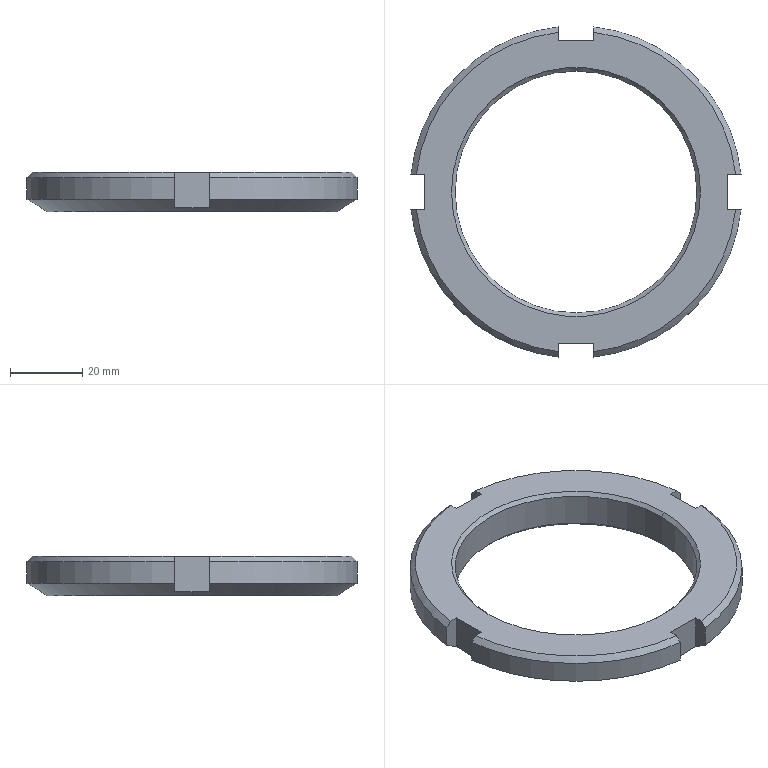Part | SolidWorks | features Chamfer 3, CirPattern 1, Cut 1, Extrusion 1 | 1 solid | 30 faces | box 91.477 x 91.477 x 11 mm | volume 29647 mm3 | plane 14 | cone 10 | cylinder 6 | commonest cylinder face diameters 92 x4 67 x2
STEP:
#1=CARTESIAN_POINT('',(-33.5,0.,10.));
#2=VERTEX_POINT('',#1);
#3=CARTESIAN_POINT('',(33.5,0.,10.));
#4=VERTEX_POINT('',#3);
#5=CARTESIAN_POINT('',(0.,0.,10.));
#6=DIRECTION('',(0.,0.,1.));
#7=DIRECTION('',(1.,0.,0.));
#8=AXIS2_PLACEMENT_3D('',#5,#6,#7);
#9=CIRCLE('',#8,33.5);
#10=EDGE_CURVE('',#2,#4,#9,.T.);
#11=ORIENTED_EDGE('',*,*,#10,.F.);
#12=CARTESIAN_POINT('',(-34.5,0.,11.));
#13=VERTEX_POINT('',#12);
#14=CARTESIAN_POINT('',(-33.5,0.,10.));
#15=DIRECTION('',(-0.7071,0.,0.7071));
#16=VECTOR('',#15,1000.);
#17=LINE('',#14,#16);
#18=EDGE_CURVE('',#2,#13,#17,.T.);
#19=ORIENTED_EDGE('',*,*,#18,.T.);
#20=CARTESIAN_POINT('',(34.5,0.,11.));
#21=VERTEX_POINT('',#20);
#22=CARTESIAN_POINT('',(0.,0.,11.));
#23=DIRECTION('',(0.,0.,-1.));
#24=DIRECTION('',(1.,0.,0.));
#25=AXIS2_PLACEMENT_3D('',#22,#23,#24);
#26=CIRCLE('',#25,34.5);
#27=EDGE_CURVE('',#21,#13,#26,.T.);
#28=ORIENTED_EDGE('',*,*,#27,.F.);
#29=CARTESIAN_POINT('',(33.5,0.,10.));
#30=DIRECTION('',(0.7071,0.,0.7071));
#31=VECTOR('',#30,1000.);
#32=LINE('',#29,#31);
#33=EDGE_CURVE('',#4,#21,#32,.T.);
#34=ORIENTED_EDGE('',*,*,#33,.F.);
#35=EDGE_LOOP('',(#11,#19,#28,#34));
#36=FACE_OUTER_BOUND('',#35,.T.);
#37=CARTESIAN_POINT('',(0.,0.,10.));
#38=DIRECTION('',(0.,0.,1.));
#39=DIRECTION('',(1.,0.,0.));
#40=AXIS2_PLACEMENT_3D('',#37,#38,#39);
#41=CONICAL_SURFACE('',#40,33.5,0.7854);
#42=ADVANCED_FACE('',(#36),#41,.F.);
#43=CARTESIAN_POINT('',(33.5,0.,1.));
#44=VERTEX_POINT('',#43);
#45=CARTESIAN_POINT('',(-33.5,0.,1.));
#46=VERTEX_POINT('',#45);
#47=CARTESIAN_POINT('',(0.,0.,1.));
#48=DIRECTION('',(0.,0.,-1.));
#49=DIRECTION('',(1.,0.,0.));
#50=AXIS2_PLACEMENT_3D('',#47,#48,#49);
#51=CIRCLE('',#50,33.5);
#52=EDGE_CURVE('',#44,#46,#51,.T.);
#53=ORIENTED_EDGE('',*,*,#52,.F.);
#54=CARTESIAN_POINT('',(34.5,0.,0.));
#55=VERTEX_POINT('',#54);
#56=CARTESIAN_POINT('',(34.5,0.,0.));
#57=DIRECTION('',(0.7071,0.,-0.7071));
#58=VECTOR('',#57,1000.);
#59=LINE('',#56,#58);
#60=EDGE_CURVE('',#44,#55,#59,.T.);
#61=ORIENTED_EDGE('',*,*,#60,.T.);
#62=CARTESIAN_POINT('',(-34.5,0.,0.));
#63=VERTEX_POINT('',#62);
#64=CARTESIAN_POINT('',(0.,0.,0.));
#65=DIRECTION('',(0.,0.,1.));
#66=DIRECTION('',(1.,0.,0.));
#67=AXIS2_PLACEMENT_3D('',#64,#65,#66);
#68=CIRCLE('',#67,34.5);
#69=EDGE_CURVE('',#63,#55,#68,.T.);
#70=ORIENTED_EDGE('',*,*,#69,.F.);
#71=CARTESIAN_POINT('',(-34.5,0.,0.));
#72=DIRECTION('',(-0.7071,0.,-0.7071));
#73=VECTOR('',#72,1000.);
#74=LINE('',#71,#73);
#75=EDGE_CURVE('',#46,#63,#74,.T.);
#76=ORIENTED_EDGE('',*,*,#75,.F.);
#77=EDGE_LOOP('',(#53,#61,#70,#76));
#78=FACE_OUTER_BOUND('',#77,.T.);
#79=CARTESIAN_POINT('',(0.,0.,0.));
#80=DIRECTION('',(0.,0.,-1.));
#81=DIRECTION('',(-1.,0.,0.));
#82=AXIS2_PLACEMENT_3D('',#79,#80,#81);
#83=CONICAL_SURFACE('',#82,34.5,0.7854);
#84=ADVANCED_FACE('',(#78),#83,.F.);
#85=CARTESIAN_POINT('',(-40.,0.,0.));
#86=VERTEX_POINT('',#85);
#87=CARTESIAN_POINT('',(40.,0.,0.));
#88=VERTEX_POINT('',#87);
#89=CARTESIAN_POINT('',(0.,0.,0.));
#90=DIRECTION('',(0.,0.,-1.));
#91=DIRECTION('',(1.,0.,0.));
#92=AXIS2_PLACEMENT_3D('',#89,#90,#91);
#93=CIRCLE('',#92,40.);
#94=EDGE_CURVE('',#86,#88,#93,.T.);
#95=ORIENTED_EDGE('',*,*,#94,.F.);
#96=CARTESIAN_POINT('',(-41.994,0.,1.151));
#97=VERTEX_POINT('',#96);
#98=CARTESIAN_POINT('',(-46.,0.,3.464));
#99=DIRECTION('',(-0.866,0.,0.5));
#100=VECTOR('',#99,1000.);
#101=LINE('',#98,#100);
#102=EDGE_CURVE('',#86,#97,#101,.T.);
#103=ORIENTED_EDGE('',*,*,#102,.T.);
#104=CARTESIAN_POINT('',(-41.994,4.9,1.316));
#105=VERTEX_POINT('',#104);
#106=CARTESIAN_POINT('',(-41.994,4.9,1.316));
#107=CARTESIAN_POINT('',(-41.994,3.271,1.207));
#108=CARTESIAN_POINT('',(-41.994,1.638,1.151));
#109=CARTESIAN_POINT('',(-41.994,0.,1.151));
#110=B_SPLINE_CURVE_WITH_KNOTS('',3,(#106,#107,#108,#109),.UNSPECIFIED.,.F.,.F.,(4,4),(0.0121,0.01699),.UNSPECIFIED.);
#111=EDGE_CURVE('',#105,#97,#110,.T.);
#112=ORIENTED_EDGE('',*,*,#111,.F.);
#113=CARTESIAN_POINT('',(-45.738,4.9,3.464));
#114=VERTEX_POINT('',#113);
#115=CARTESIAN_POINT('',(-45.738,4.9,3.464));
#116=CARTESIAN_POINT('',(-45.616,4.9,3.394));
#117=CARTESIAN_POINT('',(-45.494,4.9,3.324));
#118=CARTESIAN_POINT('',(-45.372,4.9,3.254));
#119=CARTESIAN_POINT('',(-44.246,4.9,2.607));
#120=CARTESIAN_POINT('',(-43.12,4.9,1.961));
#121=CARTESIAN_POINT('',(-41.994,4.9,1.316));
#122=B_SPLINE_CURVE_WITH_KNOTS('',3,(#115,#116,#117,#118,#119,#120,#121),.UNSPECIFIED.,.F.,.F.,(4,3,4),(0.009399,0.009822,0.01372),.UNSPECIFIED.);
#123=EDGE_CURVE('',#114,#105,#122,.T.);
#124=ORIENTED_EDGE('',*,*,#123,.F.);
#125=CARTESIAN_POINT('',(-4.9,45.738,3.464));
#126=VERTEX_POINT('',#125);
#127=CARTESIAN_POINT('',(0.,0.,3.464));
#128=DIRECTION('',(0.,0.,1.));
#129=DIRECTION('',(1.,0.,0.));
#130=AXIS2_PLACEMENT_3D('',#127,#128,#129);
#131=CIRCLE('',#130,46.);
#132=EDGE_CURVE('',#126,#114,#131,.T.);
#133=ORIENTED_EDGE('',*,*,#132,.F.);
#134=CARTESIAN_POINT('',(-4.9,41.994,1.316));
#135=VERTEX_POINT('',#134);
#136=CARTESIAN_POINT('',(-4.9,41.994,1.316));
#137=CARTESIAN_POINT('',(-4.9,42.117,1.386));
#138=CARTESIAN_POINT('',(-4.9,42.24,1.457));
#139=CARTESIAN_POINT('',(-4.9,42.364,1.528));
#140=CARTESIAN_POINT('',(-4.9,43.489,2.173));
#141=CARTESIAN_POINT('',(-4.9,44.613,2.818));
#142=CARTESIAN_POINT('',(-4.9,45.738,3.464));
#143=B_SPLINE_CURVE_WITH_KNOTS('',3,(#136,#137,#138,#139,#140,#141,#142),.UNSPECIFIED.,.F.,.F.,(4,3,4),(0.009396,0.009822,0.01371),.UNSPECIFIED.);
#144=EDGE_CURVE('',#135,#126,#143,.T.);
#145=ORIENTED_EDGE('',*,*,#144,.F.);
#146=CARTESIAN_POINT('',(4.9,41.994,1.316));
#147=VERTEX_POINT('',#146);
#148=CARTESIAN_POINT('',(4.9,41.994,1.316));
#149=CARTESIAN_POINT('',(3.276,41.994,1.207));
#150=CARTESIAN_POINT('',(1.647,41.994,1.151));
#151=CARTESIAN_POINT('',(-0.8038,41.994,1.151));
#152=CARTESIAN_POINT('',(-1.622,41.994,1.165));
#153=CARTESIAN_POINT('',(-3.26,41.994,1.22));
#154=CARTESIAN_POINT('',(-4.082,41.994,1.261));
#155=CARTESIAN_POINT('',(-4.9,41.994,1.316));
#156=B_SPLINE_CURVE_WITH_KNOTS('',3,(#148,#149,#150,#151,#152,#153,#154,#155),.UNSPECIFIED.,.F.,.F.,(4,2,2,4),(0.0121,0.01698,0.01942,0.02186),.UNSPECIFIED.);
#157=EDGE_CURVE('',#147,#135,#156,.T.);
#158=ORIENTED_EDGE('',*,*,#157,.F.);
#159=CARTESIAN_POINT('',(4.9,45.738,3.464));
#160=VERTEX_POINT('',#159);
#161=CARTESIAN_POINT('',(4.9,45.738,3.464));
#162=CARTESIAN_POINT('',(4.9,44.613,2.818));
#163=CARTESIAN_POINT('',(4.9,43.489,2.173));
#164=CARTESIAN_POINT('',(4.9,42.364,1.528));
#165=CARTESIAN_POINT('',(4.9,42.24,1.457));
#166=CARTESIAN_POINT('',(4.9,42.117,1.386));
#167=CARTESIAN_POINT('',(4.9,41.994,1.316));
#168=B_SPLINE_CURVE_WITH_KNOTS('',3,(#161,#162,#163,#164,#165,#166,#167),.UNSPECIFIED.,.F.,.F.,(4,3,4),(0.005931,0.009822,0.01025),.UNSPECIFIED.);
#169=EDGE_CURVE('',#160,#147,#168,.T.);
#170=ORIENTED_EDGE('',*,*,#169,.F.);
#171=CARTESIAN_POINT('',(45.738,4.9,3.464));
#172=VERTEX_POINT('',#171);
#173=CARTESIAN_POINT('',(0.,0.,3.464));
#174=DIRECTION('',(0.,0.,1.));
#175=DIRECTION('',(1.,0.,0.));
#176=AXIS2_PLACEMENT_3D('',#173,#174,#175);
#177=CIRCLE('',#176,46.);
#178=EDGE_CURVE('',#172,#160,#177,.T.);
#179=ORIENTED_EDGE('',*,*,#178,.F.);
#180=CARTESIAN_POINT('',(41.994,4.9,1.316));
#181=VERTEX_POINT('',#180);
#182=CARTESIAN_POINT('',(41.994,4.9,1.316));
#183=CARTESIAN_POINT('',(42.117,4.9,1.386));
#184=CARTESIAN_POINT('',(42.24,4.9,1.457));
#185=CARTESIAN_POINT('',(42.364,4.9,1.528));
#186=CARTESIAN_POINT('',(43.489,4.9,2.173));
#187=CARTESIAN_POINT('',(44.613,4.9,2.818));
#188=CARTESIAN_POINT('',(45.738,4.9,3.464));
#189=B_SPLINE_CURVE_WITH_KNOTS('',3,(#182,#183,#184,#185,#186,#187,#188),.UNSPECIFIED.,.F.,.F.,(4,3,4),(0.009396,0.009822,0.01371),.UNSPECIFIED.);
#190=EDGE_CURVE('',#181,#172,#189,.T.);
#191=ORIENTED_EDGE('',*,*,#190,.F.);
#192=CARTESIAN_POINT('',(41.994,0.,1.151));
#193=VERTEX_POINT('',#192);
#194=CARTESIAN_POINT('',(41.994,0.,1.151));
#195=CARTESIAN_POINT('',(41.994,1.638,1.151));
#196=CARTESIAN_POINT('',(41.994,3.271,1.207));
#197=CARTESIAN_POINT('',(41.994,4.9,1.316));
#198=B_SPLINE_CURVE_WITH_KNOTS('',3,(#194,#195,#196,#197),.UNSPECIFIED.,.F.,.F.,(4,4),(0.02432,0.02922),.UNSPECIFIED.);
#199=EDGE_CURVE('',#193,#181,#198,.T.);
#200=ORIENTED_EDGE('',*,*,#199,.F.);
#201=CARTESIAN_POINT('',(46.,0.,3.464));
#202=DIRECTION('',(0.866,0.,0.5));
#203=VECTOR('',#202,1000.);
#204=LINE('',#201,#203);
#205=EDGE_CURVE('',#88,#193,#204,.T.);
#206=ORIENTED_EDGE('',*,*,#205,.F.);
#207=EDGE_LOOP('',(#95,#103,#112,#124,#133,#145,#158,#170,#179,#191,#200,#206));
#208=FACE_OUTER_BOUND('',#207,.T.);
#209=CARTESIAN_POINT('',(0.,0.,3.464));
#210=DIRECTION('',(0.,0.,1.));
#211=DIRECTION('',(1.,0.,0.));
#212=AXIS2_PLACEMENT_3D('',#209,#210,#211);
#213=CONICAL_SURFACE('',#212,46.,1.047);
#214=ADVANCED_FACE('',(#208),#213,.T.);
#215=ORIENTED_EDGE('',*,*,#10,.T.);
#216=CARTESIAN_POINT('',(33.5,0.,11.));
#217=DIRECTION('',(0.,0.,-1.));
#218=VECTOR('',#217,1000.);
#219=LINE('',#216,#218);
#220=EDGE_CURVE('',#4,#44,#219,.T.);
#221=ORIENTED_EDGE('',*,*,#220,.T.);
#222=ORIENTED_EDGE('',*,*,#52,.T.);
#223=CARTESIAN_POINT('',(-33.5,0.,11.));
#224=DIRECTION('',(0.,0.,-1.));
#225=VECTOR('',#224,1000.);
#226=LINE('',#223,#225);
#227=EDGE_CURVE('',#2,#46,#226,.T.);
#228=ORIENTED_EDGE('',*,*,#227,.F.);
#229=EDGE_LOOP('',(#215,#221,#222,#228));
#230=FACE_OUTER_BOUND('',#229,.T.);
#231=CARTESIAN_POINT('',(0.,0.,11.));
#232=DIRECTION('',(0.,0.,-1.));
#233=DIRECTION('',(-1.,0.,0.));
#234=AXIS2_PLACEMENT_3D('',#231,#232,#233);
#235=CYLINDRICAL_SURFACE('',#234,33.5);
#236=ADVANCED_FACE('',(#230),#235,.F.);
#237=CARTESIAN_POINT('',(4.9,45.738,9.5));
#238=VERTEX_POINT('',#237);
#239=CARTESIAN_POINT('',(45.738,4.9,9.5));
#240=VERTEX_POINT('',#239);
#241=CARTESIAN_POINT('',(0.,0.,9.5));
#242=DIRECTION('',(0.,0.,-1.));
#243=DIRECTION('',(1.,0.,0.));
#244=AXIS2_PLACEMENT_3D('',#241,#242,#243);
#245=CIRCLE('',#244,46.);
#246=EDGE_CURVE('',#238,#240,#245,.T.);
#247=ORIENTED_EDGE('',*,*,#246,.T.);
#248=CARTESIAN_POINT('',(45.738,4.9,11.));
#249=DIRECTION('',(0.,0.,-1.));
#250=VECTOR('',#249,1000.);
#251=LINE('',#248,#250);
#252=EDGE_CURVE('',#240,#172,#251,.T.);
#253=ORIENTED_EDGE('',*,*,#252,.T.);
#254=ORIENTED_EDGE('',*,*,#178,.T.);
#255=CARTESIAN_POINT('',(4.9,45.738,11.));
#256=DIRECTION('',(0.,0.,1.));
#257=VECTOR('',#256,1000.);
#258=LINE('',#255,#257);
#259=EDGE_CURVE('',#160,#238,#258,.T.);
#260=ORIENTED_EDGE('',*,*,#259,.T.);
#261=EDGE_LOOP('',(#247,#253,#254,#260));
#262=FACE_OUTER_BOUND('',#261,.T.);
#263=CARTESIAN_POINT('',(0.,0.,11.));
#264=DIRECTION('',(0.,0.,-1.));
#265=DIRECTION('',(-1.,0.,0.));
#266=AXIS2_PLACEMENT_3D('',#263,#264,#265);
#267=CYLINDRICAL_SURFACE('',#266,46.);
#268=ADVANCED_FACE('',(#262),#267,.T.);
#269=CARTESIAN_POINT('',(44.229,4.9,11.));
#270=VERTEX_POINT('',#269);
#271=CARTESIAN_POINT('',(45.738,4.9,9.5));
#272=CARTESIAN_POINT('',(45.405,4.9,9.831));
#273=CARTESIAN_POINT('',(45.072,4.9,10.162));
#274=CARTESIAN_POINT('',(44.739,4.9,10.493));
#275=CARTESIAN_POINT('',(44.569,4.9,10.662));
#276=CARTESIAN_POINT('',(44.399,4.9,10.831));
#277=CARTESIAN_POINT('',(44.229,4.9,11.));
#278=B_SPLINE_CURVE_WITH_KNOTS('',3,(#271,#272,#273,#274,#275,#276,#277),.UNSPECIFIED.,.F.,.F.,(4,3,4),(0.007091,0.0085,0.009219),.UNSPECIFIED.);
#279=EDGE_CURVE('',#240,#270,#278,.T.);
#280=ORIENTED_EDGE('',*,*,#279,.F.);
#281=ORIENTED_EDGE('',*,*,#246,.F.);
#282=CARTESIAN_POINT('',(4.9,44.229,11.));
#283=VERTEX_POINT('',#282);
#284=CARTESIAN_POINT('',(4.9,44.229,11.));
#285=CARTESIAN_POINT('',(4.9,44.399,10.831));
#286=CARTESIAN_POINT('',(4.9,44.569,10.662));
#287=CARTESIAN_POINT('',(4.9,44.739,10.493));
#288=CARTESIAN_POINT('',(4.9,45.072,10.162));
#289=CARTESIAN_POINT('',(4.9,45.405,9.831));
#290=CARTESIAN_POINT('',(4.9,45.738,9.5));
#291=B_SPLINE_CURVE_WITH_KNOTS('',3,(#284,#285,#286,#287,#288,#289,#290),.UNSPECIFIED.,.F.,.F.,(4,3,4),(0.007781,0.0085,0.009909),.UNSPECIFIED.);
#292=EDGE_CURVE('',#283,#238,#291,.T.);
#293=ORIENTED_EDGE('',*,*,#292,.F.);
#294=CARTESIAN_POINT('',(0.,0.,11.));
#295=DIRECTION('',(0.,0.,1.));
#296=DIRECTION('',(1.,0.,0.));
#297=AXIS2_PLACEMENT_3D('',#294,#295,#296);
#298=CIRCLE('',#297,44.5);
#299=EDGE_CURVE('',#270,#283,#298,.T.);
#300=ORIENTED_EDGE('',*,*,#299,.F.);
#301=EDGE_LOOP('',(#280,#281,#293,#300));
#302=FACE_OUTER_BOUND('',#301,.T.);
#303=CARTESIAN_POINT('',(0.,0.,11.));
#304=DIRECTION('',(0.,0.,-1.));
#305=DIRECTION('',(-1.,0.,0.));
#306=AXIS2_PLACEMENT_3D('',#303,#304,#305);
#307=CONICAL_SURFACE('',#306,44.5,0.7854);
#308=ADVANCED_FACE('',(#302),#307,.T.);
#309=CARTESIAN_POINT('',(-45.738,4.9,9.5));
#310=VERTEX_POINT('',#309);
#311=CARTESIAN_POINT('',(-4.9,45.738,9.5));
#312=VERTEX_POINT('',#311);
#313=CARTESIAN_POINT('',(0.,0.,9.5));
#314=DIRECTION('',(0.,0.,-1.));
#315=DIRECTION('',(1.,0.,0.));
#316=AXIS2_PLACEMENT_3D('',#313,#314,#315);
#317=CIRCLE('',#316,46.);
#318=EDGE_CURVE('',#310,#312,#317,.T.);
#319=ORIENTED_EDGE('',*,*,#318,.T.);
#320=CARTESIAN_POINT('',(-4.9,45.738,11.));
#321=DIRECTION('',(0.,0.,-1.));
#322=VECTOR('',#321,1000.);
#323=LINE('',#320,#322);
#324=EDGE_CURVE('',#312,#126,#323,.T.);
#325=ORIENTED_EDGE('',*,*,#324,.T.);
#326=ORIENTED_EDGE('',*,*,#132,.T.);
#327=CARTESIAN_POINT('',(-45.738,4.9,11.));
#328=DIRECTION('',(0.,0.,1.));
#329=VECTOR('',#328,1000.);
#330=LINE('',#327,#329);
#331=EDGE_CURVE('',#114,#310,#330,.T.);
#332=ORIENTED_EDGE('',*,*,#331,.T.);
#333=EDGE_LOOP('',(#319,#325,#326,#332));
#334=FACE_OUTER_BOUND('',#333,.T.);
#335=CARTESIAN_POINT('',(0.,0.,11.));
#336=DIRECTION('',(0.,0.,-1.));
#337=DIRECTION('',(-1.,0.,0.));
#338=AXIS2_PLACEMENT_3D('',#335,#336,#337);
#339=CYLINDRICAL_SURFACE('',#338,46.);
#340=ADVANCED_FACE('',(#334),#339,.T.);
#341=CARTESIAN_POINT('',(-4.9,44.229,11.));
#342=VERTEX_POINT('',#341);
#343=CARTESIAN_POINT('',(-4.9,45.738,9.5));
#344=CARTESIAN_POINT('',(-4.9,45.405,9.831));
#345=CARTESIAN_POINT('',(-4.9,45.072,10.162));
#346=CARTESIAN_POINT('',(-4.9,44.739,10.493));
#347=CARTESIAN_POINT('',(-4.9,44.569,10.662));
#348=CARTESIAN_POINT('',(-4.9,44.399,10.831));
#349=CARTESIAN_POINT('',(-4.9,44.229,11.));
#350=B_SPLINE_CURVE_WITH_KNOTS('',3,(#343,#344,#345,#346,#347,#348,#349),.UNSPECIFIED.,.F.,.F.,(4,3,4),(0.007091,0.0085,0.009219),.UNSPECIFIED.);
#351=EDGE_CURVE('',#312,#342,#350,.T.);
#352=ORIENTED_EDGE('',*,*,#351,.F.);
#353=ORIENTED_EDGE('',*,*,#318,.F.);
#354=CARTESIAN_POINT('',(-44.229,4.9,11.));
#355=VERTEX_POINT('',#354);
#356=CARTESIAN_POINT('',(-44.229,4.9,11.));
#357=CARTESIAN_POINT('',(-44.567,4.9,10.664));
#358=CARTESIAN_POINT('',(-44.905,4.9,10.328));
#359=CARTESIAN_POINT('',(-45.243,4.9,9.992));
#360=CARTESIAN_POINT('',(-45.408,4.9,9.828));
#361=CARTESIAN_POINT('',(-45.573,4.9,9.664));
#362=CARTESIAN_POINT('',(-45.738,4.9,9.5));
#363=B_SPLINE_CURVE_WITH_KNOTS('',3,(#356,#357,#358,#359,#360,#361,#362),.UNSPECIFIED.,.F.,.F.,(4,3,4),(0.007071,0.0085,0.009198),.UNSPECIFIED.);
#364=EDGE_CURVE('',#355,#310,#363,.T.);
#365=ORIENTED_EDGE('',*,*,#364,.F.);
#366=CARTESIAN_POINT('',(0.,0.,11.));
#367=DIRECTION('',(0.,0.,1.));
#368=DIRECTION('',(1.,0.,0.));
#369=AXIS2_PLACEMENT_3D('',#366,#367,#368);
#370=CIRCLE('',#369,44.5);
#371=EDGE_CURVE('',#342,#355,#370,.T.);
#372=ORIENTED_EDGE('',*,*,#371,.F.);
#373=EDGE_LOOP('',(#352,#353,#365,#372));
#374=FACE_OUTER_BOUND('',#373,.T.);
#375=CARTESIAN_POINT('',(0.,0.,11.));
#376=DIRECTION('',(0.,0.,-1.));
#377=DIRECTION('',(-1.,0.,0.));
#378=AXIS2_PLACEMENT_3D('',#375,#376,#377);
#379=CONICAL_SURFACE('',#378,44.5,0.7854);
#380=ADVANCED_FACE('',(#374),#379,.T.);
#381=CARTESIAN_POINT('',(-4.9,-45.738,9.5));
#382=VERTEX_POINT('',#381);
#383=CARTESIAN_POINT('',(-45.738,-4.9,9.5));
#384=VERTEX_POINT('',#383);
#385=CARTESIAN_POINT('',(0.,0.,9.5));
#386=DIRECTION('',(0.,0.,-1.));
#387=DIRECTION('',(1.,0.,0.));
#388=AXIS2_PLACEMENT_3D('',#385,#386,#387);
#389=CIRCLE('',#388,46.);
#390=EDGE_CURVE('',#382,#384,#389,.T.);
#391=ORIENTED_EDGE('',*,*,#390,.T.);
#392=CARTESIAN_POINT('',(-45.738,-4.9,3.464));
#393=VERTEX_POINT('',#392);
#394=CARTESIAN_POINT('',(-45.738,-4.9,11.));
#395=DIRECTION('',(0.,0.,-1.));
#396=VECTOR('',#395,1000.);
#397=LINE('',#394,#396);
#398=EDGE_CURVE('',#384,#393,#397,.T.);
#399=ORIENTED_EDGE('',*,*,#398,.T.);
#400=CARTESIAN_POINT('',(-4.9,-45.738,3.464));
#401=VERTEX_POINT('',#400);
#402=CARTESIAN_POINT('',(0.,0.,3.464));
#403=DIRECTION('',(0.,0.,1.));
#404=DIRECTION('',(1.,0.,0.));
#405=AXIS2_PLACEMENT_3D('',#402,#403,#404);
#406=CIRCLE('',#405,46.);
#407=EDGE_CURVE('',#393,#401,#406,.T.);
#408=ORIENTED_EDGE('',*,*,#407,.T.);
#409=CARTESIAN_POINT('',(-4.9,-45.738,11.));
#410=DIRECTION('',(0.,0.,1.));
#411=VECTOR('',#410,1000.);
#412=LINE('',#409,#411);
#413=EDGE_CURVE('',#401,#382,#412,.T.);
#414=ORIENTED_EDGE('',*,*,#413,.T.);
#415=EDGE_LOOP('',(#391,#399,#408,#414));
#416=FACE_OUTER_BOUND('',#415,.T.);
#417=CARTESIAN_POINT('',(0.,0.,11.));
#418=DIRECTION('',(0.,0.,-1.));
#419=DIRECTION('',(-1.,0.,0.));
#420=AXIS2_PLACEMENT_3D('',#417,#418,#419);
#421=CYLINDRICAL_SURFACE('',#420,46.);
#422=ADVANCED_FACE('',(#416),#421,.T.);
#423=CARTESIAN_POINT('',(-44.229,-4.9,11.));
#424=VERTEX_POINT('',#423);
#425=CARTESIAN_POINT('',(-45.738,-4.9,9.5));
#426=CARTESIAN_POINT('',(-45.573,-4.9,9.664));
#427=CARTESIAN_POINT('',(-45.408,-4.9,9.828));
#428=CARTESIAN_POINT('',(-45.243,-4.9,9.992));
#429=CARTESIAN_POINT('',(-44.905,-4.9,10.328));
#430=CARTESIAN_POINT('',(-44.567,-4.9,10.664));
#431=CARTESIAN_POINT('',(-44.229,-4.9,11.));
#432=B_SPLINE_CURVE_WITH_KNOTS('',3,(#425,#426,#427,#428,#429,#430,#431),.UNSPECIFIED.,.F.,.F.,(4,3,4),(0.007802,0.0085,0.009929),.UNSPECIFIED.);
#433=EDGE_CURVE('',#384,#424,#432,.T.);
#434=ORIENTED_EDGE('',*,*,#433,.F.);
#435=ORIENTED_EDGE('',*,*,#390,.F.);
#436=CARTESIAN_POINT('',(-4.9,-44.229,11.));
#437=VERTEX_POINT('',#436);
#438=CARTESIAN_POINT('',(-4.9,-44.229,11.));
#439=CARTESIAN_POINT('',(-4.9,-44.567,10.664));
#440=CARTESIAN_POINT('',(-4.9,-44.905,10.328));
#441=CARTESIAN_POINT('',(-4.9,-45.243,9.992));
#442=CARTESIAN_POINT('',(-4.9,-45.408,9.828));
#443=CARTESIAN_POINT('',(-4.9,-45.573,9.664));
#444=CARTESIAN_POINT('',(-4.9,-45.738,9.5));
#445=B_SPLINE_CURVE_WITH_KNOTS('',3,(#438,#439,#440,#441,#442,#443,#444),.UNSPECIFIED.,.F.,.F.,(4,3,4),(0.007071,0.0085,0.009198),.UNSPECIFIED.);
#446=EDGE_CURVE('',#437,#382,#445,.T.);
#447=ORIENTED_EDGE('',*,*,#446,.F.);
#448=CARTESIAN_POINT('',(0.,0.,11.));
#449=DIRECTION('',(0.,0.,1.));
#450=DIRECTION('',(1.,0.,0.));
#451=AXIS2_PLACEMENT_3D('',#448,#449,#450);
#452=CIRCLE('',#451,44.5);
#453=EDGE_CURVE('',#424,#437,#452,.T.);
#454=ORIENTED_EDGE('',*,*,#453,.F.);
#455=EDGE_LOOP('',(#434,#435,#447,#454));
#456=FACE_OUTER_BOUND('',#455,.T.);
#457=CARTESIAN_POINT('',(0.,0.,11.));
#458=DIRECTION('',(0.,0.,-1.));
#459=DIRECTION('',(-1.,0.,0.));
#460=AXIS2_PLACEMENT_3D('',#457,#458,#459);
#461=CONICAL_SURFACE('',#460,44.5,0.7854);
#462=ADVANCED_FACE('',(#456),#461,.T.);
#463=ORIENTED_EDGE('',*,*,#27,.T.);
#464=CARTESIAN_POINT('',(0.,0.,11.));
#465=DIRECTION('',(0.,0.,-1.));
#466=DIRECTION('',(1.,0.,0.));
#467=AXIS2_PLACEMENT_3D('',#464,#465,#466);
#468=CIRCLE('',#467,34.5);
#469=EDGE_CURVE('',#13,#21,#468,.T.);
#470=ORIENTED_EDGE('',*,*,#469,.T.);
#471=EDGE_LOOP('',(#463,#470));
#472=FACE_BOUND('',#471,.T.);
#473=CARTESIAN_POINT('',(41.994,4.9,11.));
#474=VERTEX_POINT('',#473);
#475=CARTESIAN_POINT('',(41.994,4.9,11.));
#476=DIRECTION('',(-1.,0.,0.));
#477=VECTOR('',#476,1000.);
#478=LINE('',#475,#477);
#479=EDGE_CURVE('',#270,#474,#478,.T.);
#480=ORIENTED_EDGE('',*,*,#479,.F.);
#481=ORIENTED_EDGE('',*,*,#299,.T.);
#482=CARTESIAN_POINT('',(4.9,41.994,11.));
#483=VERTEX_POINT('',#482);
#484=CARTESIAN_POINT('',(4.9,41.994,11.));
#485=DIRECTION('',(0.,1.,0.));
#486=VECTOR('',#485,1000.);
#487=LINE('',#484,#486);
#488=EDGE_CURVE('',#483,#283,#487,.T.);
#489=ORIENTED_EDGE('',*,*,#488,.F.);
#490=CARTESIAN_POINT('',(-4.9,41.994,11.));
#491=VERTEX_POINT('',#490);
#492=CARTESIAN_POINT('',(4.9,41.994,11.));
#493=DIRECTION('',(1.,0.,0.));
#494=VECTOR('',#493,1000.);
#495=LINE('',#492,#494);
#496=EDGE_CURVE('',#491,#483,#495,.T.);
#497=ORIENTED_EDGE('',*,*,#496,.F.);
#498=CARTESIAN_POINT('',(-4.9,41.994,11.));
#499=DIRECTION('',(0.,-1.,0.));
#500=VECTOR('',#499,1000.);
#501=LINE('',#498,#500);
#502=EDGE_CURVE('',#342,#491,#501,.T.);
#503=ORIENTED_EDGE('',*,*,#502,.F.);
#504=ORIENTED_EDGE('',*,*,#371,.T.);
#505=CARTESIAN_POINT('',(-41.994,4.9,11.));
#506=VERTEX_POINT('',#505);
#507=CARTESIAN_POINT('',(-41.994,4.9,11.));
#508=DIRECTION('',(-1.,0.,0.));
#509=VECTOR('',#508,1000.);
#510=LINE('',#507,#509);
#511=EDGE_CURVE('',#506,#355,#510,.T.);
#512=ORIENTED_EDGE('',*,*,#511,.F.);
#513=CARTESIAN_POINT('',(-41.994,-4.9,11.));
#514=VERTEX_POINT('',#513);
#515=CARTESIAN_POINT('',(-41.994,4.9,11.));
#516=DIRECTION('',(0.,1.,0.));
#517=VECTOR('',#516,1000.);
#518=LINE('',#515,#517);
#519=EDGE_CURVE('',#514,#506,#518,.T.);
#520=ORIENTED_EDGE('',*,*,#519,.F.);
#521=CARTESIAN_POINT('',(-41.994,-4.9,11.));
#522=DIRECTION('',(1.,0.,0.));
#523=VECTOR('',#522,1000.);
#524=LINE('',#521,#523);
#525=EDGE_CURVE('',#424,#514,#524,.T.);
#526=ORIENTED_EDGE('',*,*,#525,.F.);
#527=ORIENTED_EDGE('',*,*,#453,.T.);
#528=CARTESIAN_POINT('',(-4.9,-41.994,11.));
#529=VERTEX_POINT('',#528);
#530=CARTESIAN_POINT('',(-4.9,-41.994,11.));
#531=DIRECTION('',(0.,-1.,0.));
#532=VECTOR('',#531,1000.);
#533=LINE('',#530,#532);
#534=EDGE_CURVE('',#529,#437,#533,.T.);
#535=ORIENTED_EDGE('',*,*,#534,.F.);
#536=CARTESIAN_POINT('',(4.9,-41.994,11.));
#537=VERTEX_POINT('',#536);
#538=CARTESIAN_POINT('',(-4.9,-41.994,11.));
#539=DIRECTION('',(-1.,0.,0.));
#540=VECTOR('',#539,1000.);
#541=LINE('',#538,#540);
#542=EDGE_CURVE('',#537,#529,#541,.T.);
#543=ORIENTED_EDGE('',*,*,#542,.F.);
#544=CARTESIAN_POINT('',(4.9,-44.229,11.));
#545=VERTEX_POINT('',#544);
#546=CARTESIAN_POINT('',(4.9,-41.994,11.));
#547=DIRECTION('',(0.,1.,0.));
#548=VECTOR('',#547,1000.);
#549=LINE('',#546,#548);
#550=EDGE_CURVE('',#545,#537,#549,.T.);
#551=ORIENTED_EDGE('',*,*,#550,.F.);
#552=CARTESIAN_POINT('',(44.229,-4.9,11.));
#553=VERTEX_POINT('',#552);
#554=CARTESIAN_POINT('',(0.,0.,11.));
#555=DIRECTION('',(0.,0.,1.));
#556=DIRECTION('',(1.,0.,0.));
#557=AXIS2_PLACEMENT_3D('',#554,#555,#556);
#558=CIRCLE('',#557,44.5);
#559=EDGE_CURVE('',#545,#553,#558,.T.);
#560=ORIENTED_EDGE('',*,*,#559,.T.);
#561=CARTESIAN_POINT('',(41.994,-4.9,11.));
#562=VERTEX_POINT('',#561);
#563=CARTESIAN_POINT('',(41.994,-4.9,11.));
#564=DIRECTION('',(1.,0.,0.));
#565=VECTOR('',#564,1000.);
#566=LINE('',#563,#565);
#567=EDGE_CURVE('',#562,#553,#566,.T.);
#568=ORIENTED_EDGE('',*,*,#567,.F.);
#569=CARTESIAN_POINT('',(41.994,-4.9,11.));
#570=DIRECTION('',(0.,-1.,0.));
#571=VECTOR('',#570,1000.);
#572=LINE('',#569,#571);
#573=EDGE_CURVE('',#474,#562,#572,.T.);
#574=ORIENTED_EDGE('',*,*,#573,.F.);
#575=EDGE_LOOP('',(#480,#481,#489,#497,#503,#504,#512,#520,#526,#527,#535,#543,#551,#560,#568,#574));
#576=FACE_OUTER_BOUND('',#575,.T.);
#577=CARTESIAN_POINT('',(0.,0.,11.));
#578=DIRECTION('',(0.,0.,1.));
#579=DIRECTION('',(1.,0.,0.));
#580=AXIS2_PLACEMENT_3D('',#577,#578,#579);
#581=PLANE('',#580);
#582=ADVANCED_FACE('',(#472,#576),#581,.T.);
#583=ORIENTED_EDGE('',*,*,#69,.T.);
#584=CARTESIAN_POINT('',(0.,0.,0.));
#585=DIRECTION('',(0.,0.,1.));
#586=DIRECTION('',(1.,0.,0.));
#587=AXIS2_PLACEMENT_3D('',#584,#585,#586);
#588=CIRCLE('',#587,34.5);
#589=EDGE_CURVE('',#55,#63,#588,.T.);
#590=ORIENTED_EDGE('',*,*,#589,.T.);
#591=EDGE_LOOP('',(#583,#590));
#592=FACE_BOUND('',#591,.T.);
#593=CARTESIAN_POINT('',(0.,0.,0.));
#594=DIRECTION('',(0.,0.,-1.));
#595=DIRECTION('',(1.,0.,0.));
#596=AXIS2_PLACEMENT_3D('',#593,#594,#595);
#597=CIRCLE('',#596,40.);
#598=EDGE_CURVE('',#88,#86,#597,.T.);
#599=ORIENTED_EDGE('',*,*,#598,.T.);
#600=ORIENTED_EDGE('',*,*,#94,.T.);
#601=EDGE_LOOP('',(#599,#600));
#602=FACE_OUTER_BOUND('',#601,.T.);
#603=CARTESIAN_POINT('',(0.,0.,0.));
#604=DIRECTION('',(0.,0.,1.));
#605=DIRECTION('',(1.,0.,0.));
#606=AXIS2_PLACEMENT_3D('',#603,#604,#605);
#607=PLANE('',#606);
#608=ADVANCED_FACE('',(#592,#602),#607,.F.);
#609=CARTESIAN_POINT('',(4.9,-45.738,3.464));
#610=VERTEX_POINT('',#609);
#611=CARTESIAN_POINT('',(45.738,-4.9,3.464));
#612=VERTEX_POINT('',#611);
#613=CARTESIAN_POINT('',(0.,0.,3.464));
#614=DIRECTION('',(0.,0.,1.));
#615=DIRECTION('',(1.,0.,0.));
#616=AXIS2_PLACEMENT_3D('',#613,#614,#615);
#617=CIRCLE('',#616,46.);
#618=EDGE_CURVE('',#610,#612,#617,.T.);
#619=ORIENTED_EDGE('',*,*,#618,.T.);
#620=CARTESIAN_POINT('',(45.738,-4.9,9.5));
#621=VERTEX_POINT('',#620);
#622=CARTESIAN_POINT('',(45.738,-4.9,11.));
#623=DIRECTION('',(0.,0.,1.));
#624=VECTOR('',#623,1000.);
#625=LINE('',#622,#624);
#626=EDGE_CURVE('',#612,#621,#625,.T.);
#627=ORIENTED_EDGE('',*,*,#626,.T.);
#628=CARTESIAN_POINT('',(4.9,-45.738,9.5));
#629=VERTEX_POINT('',#628);
#630=CARTESIAN_POINT('',(0.,0.,9.5));
#631=DIRECTION('',(0.,0.,-1.));
#632=DIRECTION('',(1.,0.,0.));
#633=AXIS2_PLACEMENT_3D('',#630,#631,#632);
#634=CIRCLE('',#633,46.);
#635=EDGE_CURVE('',#621,#629,#634,.T.);
#636=ORIENTED_EDGE('',*,*,#635,.T.);
#637=CARTESIAN_POINT('',(4.9,-45.738,11.));
#638=DIRECTION('',(0.,0.,-1.));
#639=VECTOR('',#638,1000.);
#640=LINE('',#637,#639);
#641=EDGE_CURVE('',#629,#610,#640,.T.);
#642=ORIENTED_EDGE('',*,*,#641,.T.);
#643=EDGE_LOOP('',(#619,#627,#636,#642));
#644=FACE_OUTER_BOUND('',#643,.T.);
#645=CARTESIAN_POINT('',(0.,0.,11.));
#646=DIRECTION('',(0.,0.,-1.));
#647=DIRECTION('',(-1.,0.,0.));
#648=AXIS2_PLACEMENT_3D('',#645,#646,#647);
#649=CYLINDRICAL_SURFACE('',#648,46.);
#650=ADVANCED_FACE('',(#644),#649,.T.);
#651=ORIENTED_EDGE('',*,*,#220,.F.);
#652=CARTESIAN_POINT('',(0.,0.,10.));
#653=DIRECTION('',(0.,0.,1.));
#654=DIRECTION('',(1.,0.,0.));
#655=AXIS2_PLACEMENT_3D('',#652,#653,#654);
#656=CIRCLE('',#655,33.5);
#657=EDGE_CURVE('',#4,#2,#656,.T.);
#658=ORIENTED_EDGE('',*,*,#657,.T.);
#659=ORIENTED_EDGE('',*,*,#227,.T.);
#660=CARTESIAN_POINT('',(0.,0.,1.));
#661=DIRECTION('',(0.,0.,-1.));
#662=DIRECTION('',(1.,0.,0.));
#663=AXIS2_PLACEMENT_3D('',#660,#661,#662);
#664=CIRCLE('',#663,33.5);
#665=EDGE_CURVE('',#46,#44,#664,.T.);
#666=ORIENTED_EDGE('',*,*,#665,.T.);
#667=EDGE_LOOP('',(#651,#658,#659,#666));
#668=FACE_OUTER_BOUND('',#667,.T.);
#669=CARTESIAN_POINT('',(0.,0.,11.));
#670=DIRECTION('',(0.,0.,-1.));
#671=DIRECTION('',(-1.,0.,0.));
#672=AXIS2_PLACEMENT_3D('',#669,#670,#671);
#673=CYLINDRICAL_SURFACE('',#672,33.5);
#674=ADVANCED_FACE('',(#668),#673,.F.);
#675=CARTESIAN_POINT('',(44.229,-4.9,11.));
#676=CARTESIAN_POINT('',(44.399,-4.9,10.831));
#677=CARTESIAN_POINT('',(44.569,-4.9,10.662));
#678=CARTESIAN_POINT('',(44.739,-4.9,10.493));
#679=CARTESIAN_POINT('',(45.072,-4.9,10.162));
#680=CARTESIAN_POINT('',(45.405,-4.9,9.831));
#681=CARTESIAN_POINT('',(45.738,-4.9,9.5));
#682=B_SPLINE_CURVE_WITH_KNOTS('',3,(#675,#676,#677,#678,#679,#680,#681),.UNSPECIFIED.,.F.,.F.,(4,3,4),(0.007781,0.0085,0.009909),.UNSPECIFIED.);
#683=EDGE_CURVE('',#553,#621,#682,.T.);
#684=ORIENTED_EDGE('',*,*,#683,.F.);
#685=ORIENTED_EDGE('',*,*,#559,.F.);
#686=CARTESIAN_POINT('',(4.9,-45.738,9.5));
#687=CARTESIAN_POINT('',(4.9,-45.573,9.664));
#688=CARTESIAN_POINT('',(4.9,-45.408,9.828));
#689=CARTESIAN_POINT('',(4.9,-45.243,9.992));
#690=CARTESIAN_POINT('',(4.9,-44.905,10.328));
#691=CARTESIAN_POINT('',(4.9,-44.567,10.664));
#692=CARTESIAN_POINT('',(4.9,-44.229,11.));
#693=B_SPLINE_CURVE_WITH_KNOTS('',3,(#686,#687,#688,#689,#690,#691,#692),.UNSPECIFIED.,.F.,.F.,(4,3,4),(0.007802,0.0085,0.009929),.UNSPECIFIED.);
#694=EDGE_CURVE('',#629,#545,#693,.T.);
#695=ORIENTED_EDGE('',*,*,#694,.F.);
#696=ORIENTED_EDGE('',*,*,#635,.F.);
#697=EDGE_LOOP('',(#684,#685,#695,#696));
#698=FACE_OUTER_BOUND('',#697,.T.);
#699=CARTESIAN_POINT('',(0.,0.,11.));
#700=DIRECTION('',(0.,0.,-1.));
#701=DIRECTION('',(-1.,0.,0.));
#702=AXIS2_PLACEMENT_3D('',#699,#700,#701);
#703=CONICAL_SURFACE('',#702,44.5,0.7854);
#704=ADVANCED_FACE('',(#698),#703,.T.);
#705=ORIENTED_EDGE('',*,*,#102,.F.);
#706=ORIENTED_EDGE('',*,*,#598,.F.);
#707=ORIENTED_EDGE('',*,*,#205,.T.);
#708=CARTESIAN_POINT('',(41.994,-4.9,1.316));
#709=VERTEX_POINT('',#708);
#710=CARTESIAN_POINT('',(41.994,-4.9,1.316));
#711=CARTESIAN_POINT('',(41.994,-4.084,1.261));
#712=CARTESIAN_POINT('',(41.994,-3.265,1.22));
#713=CARTESIAN_POINT('',(41.994,-1.631,1.165));
#714=CARTESIAN_POINT('',(41.994,-0.8147,1.151));
#715=CARTESIAN_POINT('',(41.994,0.,1.151));
#716=B_SPLINE_CURVE_WITH_KNOTS('',3,(#710,#711,#712,#713,#714,#715),.UNSPECIFIED.,.F.,.F.,(4,2,4),(0.01944,0.02188,0.02432),.UNSPECIFIED.);
#717=EDGE_CURVE('',#709,#193,#716,.T.);
#718=ORIENTED_EDGE('',*,*,#717,.F.);
#719=CARTESIAN_POINT('',(45.738,-4.9,3.464));
#720=CARTESIAN_POINT('',(44.613,-4.9,2.818));
#721=CARTESIAN_POINT('',(43.489,-4.9,2.173));
#722=CARTESIAN_POINT('',(42.364,-4.9,1.528));
#723=CARTESIAN_POINT('',(42.24,-4.9,1.457));
#724=CARTESIAN_POINT('',(42.117,-4.9,1.386));
#725=CARTESIAN_POINT('',(41.994,-4.9,1.316));
#726=B_SPLINE_CURVE_WITH_KNOTS('',3,(#719,#720,#721,#722,#723,#724,#725),.UNSPECIFIED.,.F.,.F.,(4,3,4),(0.005931,0.009822,0.01025),.UNSPECIFIED.);
#727=EDGE_CURVE('',#612,#709,#726,.T.);
#728=ORIENTED_EDGE('',*,*,#727,.F.);
#729=ORIENTED_EDGE('',*,*,#618,.F.);
#730=CARTESIAN_POINT('',(4.9,-41.994,1.316));
#731=VERTEX_POINT('',#730);
#732=CARTESIAN_POINT('',(4.9,-41.994,1.316));
#733=CARTESIAN_POINT('',(4.9,-43.12,1.961));
#734=CARTESIAN_POINT('',(4.9,-44.246,2.607));
#735=CARTESIAN_POINT('',(4.9,-45.372,3.254));
#736=CARTESIAN_POINT('',(4.9,-45.494,3.324));
#737=CARTESIAN_POINT('',(4.9,-45.616,3.394));
#738=CARTESIAN_POINT('',(4.9,-45.738,3.464));
#739=B_SPLINE_CURVE_WITH_KNOTS('',3,(#732,#733,#734,#735,#736,#737,#738),.UNSPECIFIED.,.F.,.F.,(4,3,4),(0.005928,0.009822,0.01025),.UNSPECIFIED.);
#740=EDGE_CURVE('',#731,#610,#739,.T.);
#741=ORIENTED_EDGE('',*,*,#740,.F.);
#742=CARTESIAN_POINT('',(-4.9,-41.994,1.316));
#743=VERTEX_POINT('',#742);
#744=CARTESIAN_POINT('',(-4.9,-41.994,1.316));
#745=CARTESIAN_POINT('',(-4.082,-41.994,1.261));
#746=CARTESIAN_POINT('',(-3.26,-41.994,1.22));
#747=CARTESIAN_POINT('',(-1.622,-41.994,1.165));
#748=CARTESIAN_POINT('',(-0.8038,-41.994,1.151));
#749=CARTESIAN_POINT('',(1.647,-41.994,1.151));
#750=CARTESIAN_POINT('',(3.276,-41.994,1.207));
#751=CARTESIAN_POINT('',(4.9,-41.994,1.316));
#752=B_SPLINE_CURVE_WITH_KNOTS('',3,(#744,#745,#746,#747,#748,#749,#750,#751),.UNSPECIFIED.,.F.,.F.,(4,2,2,4),(0.01944,0.02188,0.02433,0.02922),.UNSPECIFIED.);
#753=EDGE_CURVE('',#743,#731,#752,.T.);
#754=ORIENTED_EDGE('',*,*,#753,.F.);
#755=CARTESIAN_POINT('',(-4.9,-45.738,3.464));
#756=CARTESIAN_POINT('',(-4.9,-45.616,3.394));
#757=CARTESIAN_POINT('',(-4.9,-45.494,3.324));
#758=CARTESIAN_POINT('',(-4.9,-45.372,3.254));
#759=CARTESIAN_POINT('',(-4.9,-44.246,2.607));
#760=CARTESIAN_POINT('',(-4.9,-43.12,1.961));
#761=CARTESIAN_POINT('',(-4.9,-41.994,1.316));
#762=B_SPLINE_CURVE_WITH_KNOTS('',3,(#755,#756,#757,#758,#759,#760,#761),.UNSPECIFIED.,.F.,.F.,(4,3,4),(0.009399,0.009822,0.01372),.UNSPECIFIED.);
#763=EDGE_CURVE('',#401,#743,#762,.T.);
#764=ORIENTED_EDGE('',*,*,#763,.F.);
#765=ORIENTED_EDGE('',*,*,#407,.F.);
#766=CARTESIAN_POINT('',(-41.994,-4.9,1.316));
#767=VERTEX_POINT('',#766);
#768=CARTESIAN_POINT('',(-41.994,-4.9,1.316));
#769=CARTESIAN_POINT('',(-43.12,-4.9,1.961));
#770=CARTESIAN_POINT('',(-44.246,-4.9,2.607));
#771=CARTESIAN_POINT('',(-45.372,-4.9,3.254));
#772=CARTESIAN_POINT('',(-45.494,-4.9,3.324));
#773=CARTESIAN_POINT('',(-45.616,-4.9,3.394));
#774=CARTESIAN_POINT('',(-45.738,-4.9,3.464));
#775=B_SPLINE_CURVE_WITH_KNOTS('',3,(#768,#769,#770,#771,#772,#773,#774),.UNSPECIFIED.,.F.,.F.,(4,3,4),(0.005928,0.009822,0.01025),.UNSPECIFIED.);
#776=EDGE_CURVE('',#767,#393,#775,.T.);
#777=ORIENTED_EDGE('',*,*,#776,.F.);
#778=CARTESIAN_POINT('',(-41.994,0.,1.151));
#779=CARTESIAN_POINT('',(-41.994,-0.8147,1.151));
#780=CARTESIAN_POINT('',(-41.994,-1.631,1.165));
#781=CARTESIAN_POINT('',(-41.994,-3.265,1.22));
#782=CARTESIAN_POINT('',(-41.994,-4.084,1.261));
#783=CARTESIAN_POINT('',(-41.994,-4.9,1.316));
#784=B_SPLINE_CURVE_WITH_KNOTS('',3,(#778,#779,#780,#781,#782,#783),.UNSPECIFIED.,.F.,.F.,(4,2,4),(0.01699,0.01943,0.02186),.UNSPECIFIED.);
#785=EDGE_CURVE('',#97,#767,#784,.T.);
#786=ORIENTED_EDGE('',*,*,#785,.F.);
#787=EDGE_LOOP('',(#705,#706,#707,#718,#728,#729,#741,#754,#764,#765,#777,#786));
#788=FACE_OUTER_BOUND('',#787,.T.);
#789=CARTESIAN_POINT('',(0.,0.,3.464));
#790=DIRECTION('',(0.,0.,1.));
#791=DIRECTION('',(1.,0.,0.));
#792=AXIS2_PLACEMENT_3D('',#789,#790,#791);
#793=CONICAL_SURFACE('',#792,46.,1.047);
#794=ADVANCED_FACE('',(#788),#793,.T.);
#795=ORIENTED_EDGE('',*,*,#753,.T.);
#796=CARTESIAN_POINT('',(4.9,-41.994,0.));
#797=DIRECTION('',(0.,0.,1.));
#798=VECTOR('',#797,1000.);
#799=LINE('',#796,#798);
#800=EDGE_CURVE('',#731,#537,#799,.T.);
#801=ORIENTED_EDGE('',*,*,#800,.T.);
#802=ORIENTED_EDGE('',*,*,#542,.T.);
#803=CARTESIAN_POINT('',(-4.9,-41.994,0.));
#804=DIRECTION('',(0.,0.,1.));
#805=VECTOR('',#804,1000.);
#806=LINE('',#803,#805);
#807=EDGE_CURVE('',#743,#529,#806,.T.);
#808=ORIENTED_EDGE('',*,*,#807,.F.);
#809=EDGE_LOOP('',(#795,#801,#802,#808));
#810=FACE_OUTER_BOUND('',#809,.T.);
#811=CARTESIAN_POINT('',(-4.9,-41.994,0.));
#812=DIRECTION('',(0.,1.,0.));
#813=DIRECTION('',(0.,0.,1.));
#814=AXIS2_PLACEMENT_3D('',#811,#812,#813);
#815=PLANE('',#814);
#816=ADVANCED_FACE('',(#810),#815,.F.);
#817=ORIENTED_EDGE('',*,*,#694,.T.);
#818=ORIENTED_EDGE('',*,*,#550,.T.);
#819=ORIENTED_EDGE('',*,*,#800,.F.);
#820=ORIENTED_EDGE('',*,*,#740,.T.);
#821=ORIENTED_EDGE('',*,*,#641,.F.);
#822=EDGE_LOOP('',(#817,#818,#819,#820,#821));
#823=FACE_OUTER_BOUND('',#822,.T.);
#824=CARTESIAN_POINT('',(4.9,-41.994,0.));
#825=DIRECTION('',(1.,0.,0.));
#826=DIRECTION('',(0.,1.,0.));
#827=AXIS2_PLACEMENT_3D('',#824,#825,#826);
#828=PLANE('',#827);
#829=ADVANCED_FACE('',(#823),#828,.F.);
#830=ORIENTED_EDGE('',*,*,#446,.T.);
#831=ORIENTED_EDGE('',*,*,#413,.F.);
#832=ORIENTED_EDGE('',*,*,#763,.T.);
#833=ORIENTED_EDGE('',*,*,#807,.T.);
#834=ORIENTED_EDGE('',*,*,#534,.T.);
#835=EDGE_LOOP('',(#830,#831,#832,#833,#834));
#836=FACE_OUTER_BOUND('',#835,.T.);
#837=CARTESIAN_POINT('',(-4.9,-41.994,0.));
#838=DIRECTION('',(-1.,0.,0.));
#839=DIRECTION('',(0.,-1.,0.));
#840=AXIS2_PLACEMENT_3D('',#837,#838,#839);
#841=PLANE('',#840);
#842=ADVANCED_FACE('',(#836),#841,.F.);
#843=ORIENTED_EDGE('',*,*,#111,.T.);
#844=ORIENTED_EDGE('',*,*,#785,.T.);
#845=CARTESIAN_POINT('',(-41.994,-4.9,0.));
#846=DIRECTION('',(0.,0.,1.));
#847=VECTOR('',#846,1000.);
#848=LINE('',#845,#847);
#849=EDGE_CURVE('',#767,#514,#848,.T.);
#850=ORIENTED_EDGE('',*,*,#849,.T.);
#851=ORIENTED_EDGE('',*,*,#519,.T.);
#852=CARTESIAN_POINT('',(-41.994,4.9,0.));
#853=DIRECTION('',(0.,0.,1.));
#854=VECTOR('',#853,1000.);
#855=LINE('',#852,#854);
#856=EDGE_CURVE('',#105,#506,#855,.T.);
#857=ORIENTED_EDGE('',*,*,#856,.F.);
#858=EDGE_LOOP('',(#843,#844,#850,#851,#857));
#859=FACE_OUTER_BOUND('',#858,.T.);
#860=CARTESIAN_POINT('',(-41.994,4.9,0.));
#861=DIRECTION('',(1.,0.,0.));
#862=DIRECTION('',(0.,1.,0.));
#863=AXIS2_PLACEMENT_3D('',#860,#861,#862);
#864=PLANE('',#863);
#865=ADVANCED_FACE('',(#859),#864,.F.);
#866=ORIENTED_EDGE('',*,*,#433,.T.);
#867=ORIENTED_EDGE('',*,*,#525,.T.);
#868=ORIENTED_EDGE('',*,*,#849,.F.);
#869=ORIENTED_EDGE('',*,*,#776,.T.);
#870=ORIENTED_EDGE('',*,*,#398,.F.);
#871=EDGE_LOOP('',(#866,#867,#868,#869,#870));
#872=FACE_OUTER_BOUND('',#871,.T.);
#873=CARTESIAN_POINT('',(-41.994,-4.9,0.));
#874=DIRECTION('',(0.,-1.,0.));
#875=DIRECTION('',(1.,0.,0.));
#876=AXIS2_PLACEMENT_3D('',#873,#874,#875);
#877=PLANE('',#876);
#878=ADVANCED_FACE('',(#872),#877,.F.);
#879=ORIENTED_EDGE('',*,*,#364,.T.);
#880=ORIENTED_EDGE('',*,*,#331,.F.);
#881=ORIENTED_EDGE('',*,*,#123,.T.);
#882=ORIENTED_EDGE('',*,*,#856,.T.);
#883=ORIENTED_EDGE('',*,*,#511,.T.);
#884=EDGE_LOOP('',(#879,#880,#881,#882,#883));
#885=FACE_OUTER_BOUND('',#884,.T.);
#886=CARTESIAN_POINT('',(-41.994,4.9,0.));
#887=DIRECTION('',(0.,1.,0.));
#888=DIRECTION('',(-1.,0.,0.));
#889=AXIS2_PLACEMENT_3D('',#886,#887,#888);
#890=PLANE('',#889);
#891=ADVANCED_FACE('',(#885),#890,.F.);
#892=ORIENTED_EDGE('',*,*,#157,.T.);
#893=CARTESIAN_POINT('',(-4.9,41.994,0.));
#894=DIRECTION('',(0.,0.,1.));
#895=VECTOR('',#894,1000.);
#896=LINE('',#893,#895);
#897=EDGE_CURVE('',#135,#491,#896,.T.);
#898=ORIENTED_EDGE('',*,*,#897,.T.);
#899=ORIENTED_EDGE('',*,*,#496,.T.);
#900=CARTESIAN_POINT('',(4.9,41.994,0.));
#901=DIRECTION('',(0.,0.,1.));
#902=VECTOR('',#901,1000.);
#903=LINE('',#900,#902);
#904=EDGE_CURVE('',#147,#483,#903,.T.);
#905=ORIENTED_EDGE('',*,*,#904,.F.);
#906=EDGE_LOOP('',(#892,#898,#899,#905));
#907=FACE_OUTER_BOUND('',#906,.T.);
#908=CARTESIAN_POINT('',(4.9,41.994,0.));
#909=DIRECTION('',(0.,-1.,0.));
#910=DIRECTION('',(1.,0.,0.));
#911=AXIS2_PLACEMENT_3D('',#908,#909,#910);
#912=PLANE('',#911);
#913=ADVANCED_FACE('',(#907),#912,.F.);
#914=ORIENTED_EDGE('',*,*,#351,.T.);
#915=ORIENTED_EDGE('',*,*,#502,.T.);
#916=ORIENTED_EDGE('',*,*,#897,.F.);
#917=ORIENTED_EDGE('',*,*,#144,.T.);
#918=ORIENTED_EDGE('',*,*,#324,.F.);
#919=EDGE_LOOP('',(#914,#915,#916,#917,#918));
#920=FACE_OUTER_BOUND('',#919,.T.);
#921=CARTESIAN_POINT('',(-4.9,41.994,0.));
#922=DIRECTION('',(-1.,0.,0.));
#923=DIRECTION('',(0.,-1.,0.));
#924=AXIS2_PLACEMENT_3D('',#921,#922,#923);
#925=PLANE('',#924);
#926=ADVANCED_FACE('',(#920),#925,.F.);
#927=ORIENTED_EDGE('',*,*,#292,.T.);
#928=ORIENTED_EDGE('',*,*,#259,.F.);
#929=ORIENTED_EDGE('',*,*,#169,.T.);
#930=ORIENTED_EDGE('',*,*,#904,.T.);
#931=ORIENTED_EDGE('',*,*,#488,.T.);
#932=EDGE_LOOP('',(#927,#928,#929,#930,#931));
#933=FACE_OUTER_BOUND('',#932,.T.);
#934=CARTESIAN_POINT('',(4.9,41.994,0.));
#935=DIRECTION('',(1.,0.,0.));
#936=DIRECTION('',(0.,1.,0.));
#937=AXIS2_PLACEMENT_3D('',#934,#935,#936);
#938=PLANE('',#937);
#939=ADVANCED_FACE('',(#933),#938,.F.);
#940=ORIENTED_EDGE('',*,*,#717,.T.);
#941=ORIENTED_EDGE('',*,*,#199,.T.);
#942=CARTESIAN_POINT('',(41.994,4.9,0.));
#943=DIRECTION('',(0.,0.,1.));
#944=VECTOR('',#943,1000.);
#945=LINE('',#942,#944);
#946=EDGE_CURVE('',#181,#474,#945,.T.);
#947=ORIENTED_EDGE('',*,*,#946,.T.);
#948=ORIENTED_EDGE('',*,*,#573,.T.);
#949=CARTESIAN_POINT('',(41.994,-4.9,0.));
#950=DIRECTION('',(0.,0.,1.));
#951=VECTOR('',#950,1000.);
#952=LINE('',#949,#951);
#953=EDGE_CURVE('',#709,#562,#952,.T.);
#954=ORIENTED_EDGE('',*,*,#953,.F.);
#955=EDGE_LOOP('',(#940,#941,#947,#948,#954));
#956=FACE_OUTER_BOUND('',#955,.T.);
#957=CARTESIAN_POINT('',(41.994,-4.9,0.));
#958=DIRECTION('',(-1.,0.,0.));
#959=DIRECTION('',(0.,-1.,0.));
#960=AXIS2_PLACEMENT_3D('',#957,#958,#959);
#961=PLANE('',#960);
#962=ADVANCED_FACE('',(#956),#961,.F.);
#963=ORIENTED_EDGE('',*,*,#279,.T.);
#964=ORIENTED_EDGE('',*,*,#479,.T.);
#965=ORIENTED_EDGE('',*,*,#946,.F.);
#966=ORIENTED_EDGE('',*,*,#190,.T.);
#967=ORIENTED_EDGE('',*,*,#252,.F.);
#968=EDGE_LOOP('',(#963,#964,#965,#966,#967));
#969=FACE_OUTER_BOUND('',#968,.T.);
#970=CARTESIAN_POINT('',(41.994,4.9,0.));
#971=DIRECTION('',(0.,1.,0.));
#972=DIRECTION('',(-1.,0.,0.));
#973=AXIS2_PLACEMENT_3D('',#970,#971,#972);
#974=PLANE('',#973);
#975=ADVANCED_FACE('',(#969),#974,.F.);
#976=ORIENTED_EDGE('',*,*,#683,.T.);
#977=ORIENTED_EDGE('',*,*,#626,.F.);
#978=ORIENTED_EDGE('',*,*,#727,.T.);
#979=ORIENTED_EDGE('',*,*,#953,.T.);
#980=ORIENTED_EDGE('',*,*,#567,.T.);
#981=EDGE_LOOP('',(#976,#977,#978,#979,#980));
#982=FACE_OUTER_BOUND('',#981,.T.);
#983=CARTESIAN_POINT('',(41.994,-4.9,0.));
#984=DIRECTION('',(0.,-1.,0.));
#985=DIRECTION('',(1.,0.,0.));
#986=AXIS2_PLACEMENT_3D('',#983,#984,#985);
#987=PLANE('',#986);
#988=ADVANCED_FACE('',(#982),#987,.F.);
#989=ORIENTED_EDGE('',*,*,#60,.F.);
#990=ORIENTED_EDGE('',*,*,#665,.F.);
#991=ORIENTED_EDGE('',*,*,#75,.T.);
#992=ORIENTED_EDGE('',*,*,#589,.F.);
#993=EDGE_LOOP('',(#989,#990,#991,#992));
#994=FACE_OUTER_BOUND('',#993,.T.);
#995=CARTESIAN_POINT('',(0.,0.,0.));
#996=DIRECTION('',(0.,0.,-1.));
#997=DIRECTION('',(-1.,0.,0.));
#998=AXIS2_PLACEMENT_3D('',#995,#996,#997);
#999=CONICAL_SURFACE('',#998,34.5,0.7854);
#1000=ADVANCED_FACE('',(#994),#999,.F.);
#1001=ORIENTED_EDGE('',*,*,#18,.F.);
#1002=ORIENTED_EDGE('',*,*,#657,.F.);
#1003=ORIENTED_EDGE('',*,*,#33,.T.);
#1004=ORIENTED_EDGE('',*,*,#469,.F.);
#1005=EDGE_LOOP('',(#1001,#1002,#1003,#1004));
#1006=FACE_OUTER_BOUND('',#1005,.T.);
#1007=CARTESIAN_POINT('',(0.,0.,10.));
#1008=DIRECTION('',(0.,0.,1.));
#1009=DIRECTION('',(1.,0.,0.));
#1010=AXIS2_PLACEMENT_3D('',#1007,#1008,#1009);
#1011=CONICAL_SURFACE('',#1010,33.5,0.7854);
#1012=ADVANCED_FACE('',(#1006),#1011,.F.);
#1013=CLOSED_SHELL('',(#42,#84,#214,#236,#268,#308,#340,#380,#422,#462,#582,#608,#650,#674,#704,#794,#816,#829,#842,#865,#878,#891,#913,#926,#939,#962,#975,#988,#1000,#1012));
#1014=MANIFOLD_SOLID_BREP('',#1013);
#1015=CARTESIAN_POINT('',(0.,0.,0.));
#1016=DIRECTION('',(0.,0.,1.));
#1017=DIRECTION('',(1.,0.,0.));
#1018=AXIS2_PLACEMENT_3D('',#1015,#1016,#1017);
#1019=(LENGTH_UNIT()NAMED_UNIT(*)SI_UNIT(.MILLI.,.METRE.));
#1020=UNCERTAINTY_MEASURE_WITH_UNIT(LENGTH_MEASURE(0.00001),#1019,'','');
#1021=(NAMED_UNIT(*)PLANE_ANGLE_UNIT()SI_UNIT($,.RADIAN.));
#1022=(NAMED_UNIT(*)SI_UNIT($,.STERADIAN.)SOLID_ANGLE_UNIT());
#1023=(GEOMETRIC_REPRESENTATION_CONTEXT(3)GLOBAL_UNCERTAINTY_ASSIGNED_CONTEXT((#1020))GLOBAL_UNIT_ASSIGNED_CONTEXT((#1019,#1021,#1022))REPRESENTATION_CONTEXT('',''));
#1024=ADVANCED_BREP_SHAPE_REPRESENTATION('',(#1014,#1018),#1023);